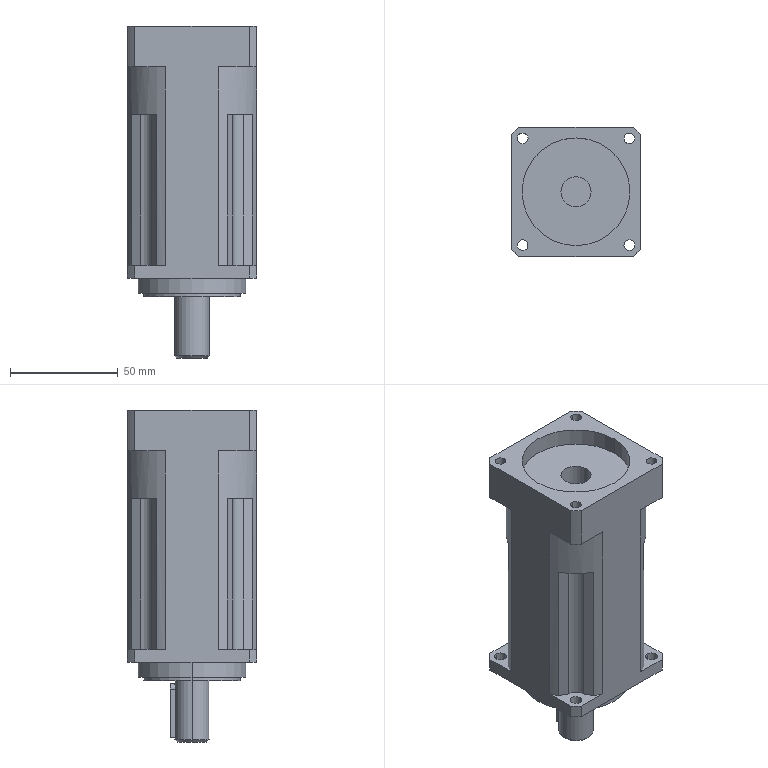Part | STEP file | AB060A-030-S2-P2 | 1 solid | 87 faces | box 60 x 60 x 154 mm | volume 369054 mm3 | cylinder 46 | plane 35 | cone 6 | commonest cylinder face diameters 5 x10 5.5 x8 80 x8 12 x4 50 x4 65 x4